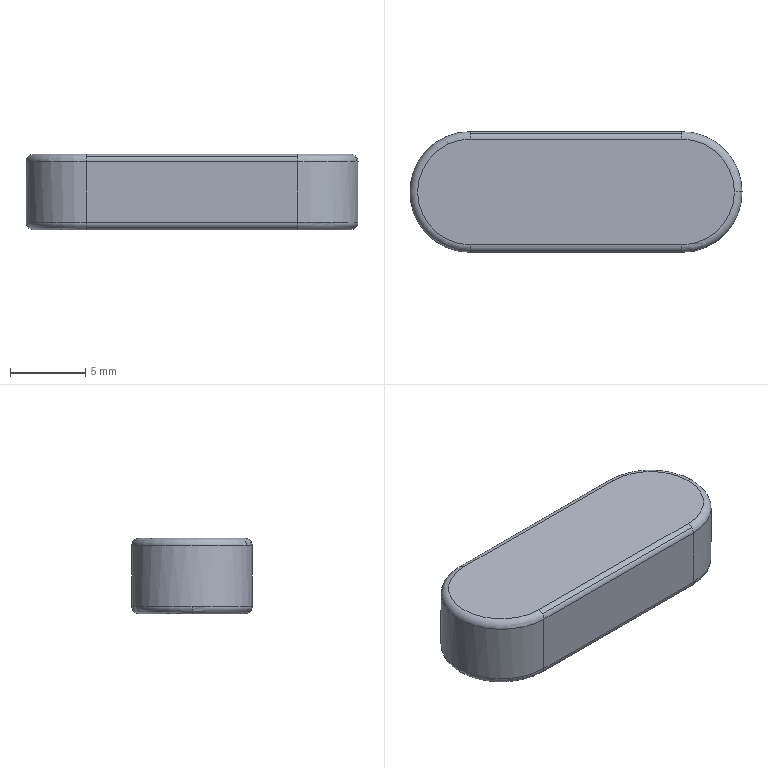Part | SolidWorks | features BaseBody 1 | 1 solid | 20 faces | box 22 x 8 x 5 mm | volume 805.702 mm3 | cylinder 10 | torus 6 | plane 4 | commonest cylinder face diameters 1 x8 8 x2
STEP:
#1=CARTESIAN_POINT('',(0.,-8.,-4.5));
#2=VERTEX_POINT('',#1);
#3=CARTESIAN_POINT('',(0.,-7.854,-4.854));
#4=VERTEX_POINT('',#3);
#5=CARTESIAN_POINT('',(0.,-7.5,-4.5));
#6=DIRECTION('',(1.,0.,0.));
#7=DIRECTION('',(0.,-1.,0.));
#8=AXIS2_PLACEMENT_3D('',#5,#6,#7);
#9=CIRCLE('',#8,0.5);
#10=EDGE_CURVE('',#2,#4,#9,.T.);
#11=ORIENTED_EDGE('',*,*,#10,.T.);
#12=CARTESIAN_POINT('',(14.,-7.854,-4.854));
#13=VERTEX_POINT('',#12);
#14=CARTESIAN_POINT('',(6.311,-7.854,-4.854));
#15=DIRECTION('',(1.,0.,0.));
#16=VECTOR('',#15,1000.);
#17=LINE('',#14,#16);
#18=EDGE_CURVE('',#4,#13,#17,.T.);
#19=ORIENTED_EDGE('',*,*,#18,.T.);
#20=CARTESIAN_POINT('',(14.,-8.,-4.5));
#21=VERTEX_POINT('',#20);
#22=CARTESIAN_POINT('',(14.,-7.5,-4.5));
#23=DIRECTION('',(-1.,0.,0.));
#24=DIRECTION('',(0.,0.,-1.));
#25=AXIS2_PLACEMENT_3D('',#22,#23,#24);
#26=CIRCLE('',#25,0.5);
#27=EDGE_CURVE('',#13,#21,#26,.T.);
#28=ORIENTED_EDGE('',*,*,#27,.T.);
#29=CARTESIAN_POINT('',(6.311,-8.,-4.5));
#30=DIRECTION('',(-1.,0.,0.));
#31=VECTOR('',#30,1000.);
#32=LINE('',#29,#31);
#33=EDGE_CURVE('',#21,#2,#32,.T.);
#34=ORIENTED_EDGE('',*,*,#33,.T.);
#35=EDGE_LOOP('',(#11,#19,#28,#34));
#36=FACE_OUTER_BOUND('',#35,.T.);
#37=CARTESIAN_POINT('',(6.311,-7.5,-4.5));
#38=DIRECTION('',(1.,0.,0.));
#39=DIRECTION('',(0.,-0.7071,-0.7071));
#40=AXIS2_PLACEMENT_3D('',#37,#38,#39);
#41=CYLINDRICAL_SURFACE('',#40,0.5);
#42=ADVANCED_FACE('',(#36),#41,.T.);
#43=CARTESIAN_POINT('',(-4.,-4.,-4.5));
#44=VERTEX_POINT('',#43);
#45=CARTESIAN_POINT('',(0.,-4.,-4.5));
#46=DIRECTION('',(0.,0.,-1.));
#47=DIRECTION('',(-1.,0.,0.));
#48=AXIS2_PLACEMENT_3D('',#45,#46,#47);
#49=CIRCLE('',#48,4.);
#50=EDGE_CURVE('',#2,#44,#49,.T.);
#51=ORIENTED_EDGE('',*,*,#50,.T.);
#52=CARTESIAN_POINT('',(-3.5,-4.,-5.));
#53=VERTEX_POINT('',#52);
#54=CARTESIAN_POINT('',(-3.5,-4.,-4.5));
#55=DIRECTION('',(0.,-1.,0.));
#56=DIRECTION('',(0.,0.,-1.));
#57=AXIS2_PLACEMENT_3D('',#54,#55,#56);
#58=CIRCLE('',#57,0.5);
#59=EDGE_CURVE('',#44,#53,#58,.T.);
#60=ORIENTED_EDGE('',*,*,#59,.T.);
#61=CARTESIAN_POINT('',(0.,-7.5,-5.));
#62=VERTEX_POINT('',#61);
#63=CARTESIAN_POINT('',(0.,-4.,-5.));
#64=DIRECTION('',(0.,0.,1.));
#65=DIRECTION('',(-1.,0.,0.));
#66=AXIS2_PLACEMENT_3D('',#63,#64,#65);
#67=CIRCLE('',#66,3.5);
#68=EDGE_CURVE('',#53,#62,#67,.T.);
#69=ORIENTED_EDGE('',*,*,#68,.T.);
#70=CARTESIAN_POINT('',(0.,-7.5,-4.5));
#71=DIRECTION('',(1.,0.,0.));
#72=DIRECTION('',(0.,-1.,0.));
#73=AXIS2_PLACEMENT_3D('',#70,#71,#72);
#74=CIRCLE('',#73,0.5);
#75=EDGE_CURVE('',#4,#62,#74,.T.);
#76=ORIENTED_EDGE('',*,*,#75,.F.);
#77=ORIENTED_EDGE('',*,*,#10,.F.);
#78=EDGE_LOOP('',(#51,#60,#69,#76,#77));
#79=FACE_OUTER_BOUND('',#78,.T.);
#80=CARTESIAN_POINT('',(0.,-4.,-4.5));
#81=DIRECTION('',(0.,0.,-1.));
#82=DIRECTION('',(-1.,0.,0.));
#83=AXIS2_PLACEMENT_3D('',#80,#81,#82);
#84=TOROIDAL_SURFACE('',#83,3.5,0.5);
#85=ADVANCED_FACE('',(#79),#84,.T.);
#86=CARTESIAN_POINT('',(14.,0.,-4.5));
#87=VERTEX_POINT('',#86);
#88=CARTESIAN_POINT('',(14.,-0.1464,-4.854));
#89=VERTEX_POINT('',#88);
#90=CARTESIAN_POINT('',(14.,-0.5,-4.5));
#91=DIRECTION('',(-1.,0.,0.));
#92=DIRECTION('',(0.,1.,0.));
#93=AXIS2_PLACEMENT_3D('',#90,#91,#92);
#94=CIRCLE('',#93,0.5);
#95=EDGE_CURVE('',#87,#89,#94,.T.);
#96=ORIENTED_EDGE('',*,*,#95,.T.);
#97=CARTESIAN_POINT('',(0.,-0.1464,-4.854));
#98=VERTEX_POINT('',#97);
#99=CARTESIAN_POINT('',(-0.6887,-0.1464,-4.854));
#100=DIRECTION('',(-1.,0.,0.));
#101=VECTOR('',#100,1000.);
#102=LINE('',#99,#101);
#103=EDGE_CURVE('',#89,#98,#102,.T.);
#104=ORIENTED_EDGE('',*,*,#103,.T.);
#105=CARTESIAN_POINT('',(0.,0.,-4.5));
#106=VERTEX_POINT('',#105);
#107=CARTESIAN_POINT('',(0.,-0.5,-4.5));
#108=DIRECTION('',(-1.,0.,0.));
#109=DIRECTION('',(0.,1.,0.));
#110=AXIS2_PLACEMENT_3D('',#107,#108,#109);
#111=CIRCLE('',#110,0.5);
#112=EDGE_CURVE('',#106,#98,#111,.T.);
#113=ORIENTED_EDGE('',*,*,#112,.F.);
#114=CARTESIAN_POINT('',(-0.6887,0.,-4.5));
#115=DIRECTION('',(1.,0.,0.));
#116=VECTOR('',#115,1000.);
#117=LINE('',#114,#116);
#118=EDGE_CURVE('',#106,#87,#117,.T.);
#119=ORIENTED_EDGE('',*,*,#118,.T.);
#120=EDGE_LOOP('',(#96,#104,#113,#119));
#121=FACE_OUTER_BOUND('',#120,.T.);
#122=CARTESIAN_POINT('',(-0.6887,-0.5,-4.5));
#123=DIRECTION('',(-1.,0.,0.));
#124=DIRECTION('',(0.,0.7071,-0.7071));
#125=AXIS2_PLACEMENT_3D('',#122,#123,#124);
#126=CYLINDRICAL_SURFACE('',#125,0.5);
#127=ADVANCED_FACE('',(#121),#126,.T.);
#128=CARTESIAN_POINT('',(0.,0.,-0.5));
#129=VERTEX_POINT('',#128);
#130=CARTESIAN_POINT('',(0.,-0.1464,-0.1464));
#131=VERTEX_POINT('',#130);
#132=CARTESIAN_POINT('',(0.,-0.5,-0.5));
#133=DIRECTION('',(1.,0.,0.));
#134=DIRECTION('',(0.,1.,0.));
#135=AXIS2_PLACEMENT_3D('',#132,#133,#134);
#136=CIRCLE('',#135,0.5);
#137=EDGE_CURVE('',#129,#131,#136,.T.);
#138=ORIENTED_EDGE('',*,*,#137,.T.);
#139=CARTESIAN_POINT('',(14.,-0.1464,-0.1464));
#140=VERTEX_POINT('',#139);
#141=CARTESIAN_POINT('',(-0.6887,-0.1464,-0.1464));
#142=DIRECTION('',(1.,0.,0.));
#143=VECTOR('',#142,1000.);
#144=LINE('',#141,#143);
#145=EDGE_CURVE('',#131,#140,#144,.T.);
#146=ORIENTED_EDGE('',*,*,#145,.T.);
#147=CARTESIAN_POINT('',(14.,0.,-0.5));
#148=VERTEX_POINT('',#147);
#149=CARTESIAN_POINT('',(14.,-0.5,-0.5));
#150=DIRECTION('',(-1.,0.,0.));
#151=DIRECTION('',(0.,0.,1.));
#152=AXIS2_PLACEMENT_3D('',#149,#150,#151);
#153=CIRCLE('',#152,0.5);
#154=EDGE_CURVE('',#140,#148,#153,.T.);
#155=ORIENTED_EDGE('',*,*,#154,.T.);
#156=CARTESIAN_POINT('',(-0.6887,0.,-0.5));
#157=DIRECTION('',(-1.,0.,0.));
#158=VECTOR('',#157,1000.);
#159=LINE('',#156,#158);
#160=EDGE_CURVE('',#148,#129,#159,.T.);
#161=ORIENTED_EDGE('',*,*,#160,.T.);
#162=EDGE_LOOP('',(#138,#146,#155,#161));
#163=FACE_OUTER_BOUND('',#162,.T.);
#164=CARTESIAN_POINT('',(-0.6887,-0.5,-0.5));
#165=DIRECTION('',(1.,0.,0.));
#166=DIRECTION('',(0.,0.7071,0.7071));
#167=AXIS2_PLACEMENT_3D('',#164,#165,#166);
#168=CYLINDRICAL_SURFACE('',#167,0.5);
#169=ADVANCED_FACE('',(#163),#168,.T.);
#170=CARTESIAN_POINT('',(14.,-8.,-0.5));
#171=VERTEX_POINT('',#170);
#172=CARTESIAN_POINT('',(14.,-7.854,-0.1464));
#173=VERTEX_POINT('',#172);
#174=CARTESIAN_POINT('',(14.,-7.5,-0.5));
#175=DIRECTION('',(-1.,0.,0.));
#176=DIRECTION('',(0.,-1.,0.));
#177=AXIS2_PLACEMENT_3D('',#174,#175,#176);
#178=CIRCLE('',#177,0.5);
#179=EDGE_CURVE('',#171,#173,#178,.T.);
#180=ORIENTED_EDGE('',*,*,#179,.T.);
#181=CARTESIAN_POINT('',(0.,-7.854,-0.1464));
#182=VERTEX_POINT('',#181);
#183=CARTESIAN_POINT('',(6.311,-7.854,-0.1464));
#184=DIRECTION('',(-1.,0.,0.));
#185=VECTOR('',#184,1000.);
#186=LINE('',#183,#185);
#187=EDGE_CURVE('',#173,#182,#186,.T.);
#188=ORIENTED_EDGE('',*,*,#187,.T.);
#189=CARTESIAN_POINT('',(0.,-8.,-0.5));
#190=VERTEX_POINT('',#189);
#191=CARTESIAN_POINT('',(0.,-7.5,-0.5));
#192=DIRECTION('',(-1.,0.,0.));
#193=DIRECTION('',(0.,-1.,0.));
#194=AXIS2_PLACEMENT_3D('',#191,#192,#193);
#195=CIRCLE('',#194,0.5);
#196=EDGE_CURVE('',#190,#182,#195,.T.);
#197=ORIENTED_EDGE('',*,*,#196,.F.);
#198=CARTESIAN_POINT('',(6.311,-8.,-0.5));
#199=DIRECTION('',(1.,0.,0.));
#200=VECTOR('',#199,1000.);
#201=LINE('',#198,#200);
#202=EDGE_CURVE('',#190,#171,#201,.T.);
#203=ORIENTED_EDGE('',*,*,#202,.T.);
#204=EDGE_LOOP('',(#180,#188,#197,#203));
#205=FACE_OUTER_BOUND('',#204,.T.);
#206=CARTESIAN_POINT('',(6.311,-7.5,-0.5));
#207=DIRECTION('',(-1.,0.,0.));
#208=DIRECTION('',(0.,-0.7071,0.7071));
#209=AXIS2_PLACEMENT_3D('',#206,#207,#208);
#210=CYLINDRICAL_SURFACE('',#209,0.5);
#211=ADVANCED_FACE('',(#205),#210,.T.);
#212=CARTESIAN_POINT('',(18.,-4.,-0.5));
#213=VERTEX_POINT('',#212);
#214=CARTESIAN_POINT('',(14.,-4.,-0.5));
#215=DIRECTION('',(0.,0.,1.));
#216=DIRECTION('',(1.,0.,0.));
#217=AXIS2_PLACEMENT_3D('',#214,#215,#216);
#218=CIRCLE('',#217,4.);
#219=EDGE_CURVE('',#171,#213,#218,.T.);
#220=ORIENTED_EDGE('',*,*,#219,.T.);
#221=CARTESIAN_POINT('',(17.5,-4.,0.));
#222=VERTEX_POINT('',#221);
#223=CARTESIAN_POINT('',(17.5,-4.,-0.5));
#224=DIRECTION('',(0.,-1.,0.));
#225=DIRECTION('',(0.,0.,-1.));
#226=AXIS2_PLACEMENT_3D('',#223,#224,#225);
#227=CIRCLE('',#226,0.5);
#228=EDGE_CURVE('',#213,#222,#227,.T.);
#229=ORIENTED_EDGE('',*,*,#228,.T.);
#230=CARTESIAN_POINT('',(14.,-7.5,0.));
#231=VERTEX_POINT('',#230);
#232=CARTESIAN_POINT('',(14.,-4.,0.));
#233=DIRECTION('',(0.,0.,-1.));
#234=DIRECTION('',(1.,0.,0.));
#235=AXIS2_PLACEMENT_3D('',#232,#233,#234);
#236=CIRCLE('',#235,3.5);
#237=EDGE_CURVE('',#222,#231,#236,.T.);
#238=ORIENTED_EDGE('',*,*,#237,.T.);
#239=CARTESIAN_POINT('',(14.,-7.5,-0.5));
#240=DIRECTION('',(-1.,0.,0.));
#241=DIRECTION('',(0.,-1.,0.));
#242=AXIS2_PLACEMENT_3D('',#239,#240,#241);
#243=CIRCLE('',#242,0.5);
#244=EDGE_CURVE('',#173,#231,#243,.T.);
#245=ORIENTED_EDGE('',*,*,#244,.F.);
#246=ORIENTED_EDGE('',*,*,#179,.F.);
#247=EDGE_LOOP('',(#220,#229,#238,#245,#246));
#248=FACE_OUTER_BOUND('',#247,.T.);
#249=CARTESIAN_POINT('',(14.,-4.,-0.5));
#250=DIRECTION('',(0.,0.,1.));
#251=DIRECTION('',(1.,0.,0.));
#252=AXIS2_PLACEMENT_3D('',#249,#250,#251);
#253=TOROIDAL_SURFACE('',#252,3.5,0.5);
#254=ADVANCED_FACE('',(#248),#253,.T.);
#255=CARTESIAN_POINT('',(14.,-7.5,-5.));
#256=VERTEX_POINT('',#255);
#257=CARTESIAN_POINT('',(14.,-7.5,-4.5));
#258=DIRECTION('',(-1.,0.,0.));
#259=DIRECTION('',(0.,0.,-1.));
#260=AXIS2_PLACEMENT_3D('',#257,#258,#259);
#261=CIRCLE('',#260,0.5);
#262=EDGE_CURVE('',#256,#13,#261,.T.);
#263=ORIENTED_EDGE('',*,*,#262,.F.);
#264=CARTESIAN_POINT('',(14.,-0.5,-5.));
#265=VERTEX_POINT('',#264);
#266=CARTESIAN_POINT('',(14.,-4.,-5.));
#267=DIRECTION('',(0.,0.,1.));
#268=DIRECTION('',(1.,0.,0.));
#269=AXIS2_PLACEMENT_3D('',#266,#267,#268);
#270=CIRCLE('',#269,3.5);
#271=EDGE_CURVE('',#256,#265,#270,.T.);
#272=ORIENTED_EDGE('',*,*,#271,.T.);
#273=CARTESIAN_POINT('',(14.,-0.5,-4.5));
#274=DIRECTION('',(-1.,0.,0.));
#275=DIRECTION('',(0.,1.,0.));
#276=AXIS2_PLACEMENT_3D('',#273,#274,#275);
#277=CIRCLE('',#276,0.5);
#278=EDGE_CURVE('',#89,#265,#277,.T.);
#279=ORIENTED_EDGE('',*,*,#278,.F.);
#280=ORIENTED_EDGE('',*,*,#95,.F.);
#281=CARTESIAN_POINT('',(14.,-4.,-4.5));
#282=DIRECTION('',(0.,0.,-1.));
#283=DIRECTION('',(1.,0.,0.));
#284=AXIS2_PLACEMENT_3D('',#281,#282,#283);
#285=CIRCLE('',#284,4.);
#286=EDGE_CURVE('',#87,#21,#285,.T.);
#287=ORIENTED_EDGE('',*,*,#286,.T.);
#288=ORIENTED_EDGE('',*,*,#27,.F.);
#289=EDGE_LOOP('',(#263,#272,#279,#280,#287,#288));
#290=FACE_OUTER_BOUND('',#289,.T.);
#291=CARTESIAN_POINT('',(14.,-4.,-4.5));
#292=DIRECTION('',(0.,0.,-1.));
#293=DIRECTION('',(-1.,0.,0.));
#294=AXIS2_PLACEMENT_3D('',#291,#292,#293);
#295=TOROIDAL_SURFACE('',#294,3.5,0.5);
#296=ADVANCED_FACE('',(#290),#295,.T.);
#297=ORIENTED_EDGE('',*,*,#50,.F.);
#298=CARTESIAN_POINT('',(0.,-8.,0.));
#299=DIRECTION('',(0.,0.,-1.));
#300=VECTOR('',#299,1000.);
#301=LINE('',#298,#300);
#302=EDGE_CURVE('',#190,#2,#301,.T.);
#303=ORIENTED_EDGE('',*,*,#302,.F.);
#304=CARTESIAN_POINT('',(0.,-4.,-0.5));
#305=DIRECTION('',(0.,0.,1.));
#306=DIRECTION('',(-1.,0.,0.));
#307=AXIS2_PLACEMENT_3D('',#304,#305,#306);
#308=CIRCLE('',#307,4.);
#309=EDGE_CURVE('',#129,#190,#308,.T.);
#310=ORIENTED_EDGE('',*,*,#309,.F.);
#311=CARTESIAN_POINT('',(0.,0.,0.));
#312=DIRECTION('',(0.,0.,-1.));
#313=VECTOR('',#312,1000.);
#314=LINE('',#311,#313);
#315=EDGE_CURVE('',#129,#106,#314,.T.);
#316=ORIENTED_EDGE('',*,*,#315,.T.);
#317=CARTESIAN_POINT('',(0.,-4.,-4.5));
#318=DIRECTION('',(0.,0.,-1.));
#319=DIRECTION('',(-1.,0.,0.));
#320=AXIS2_PLACEMENT_3D('',#317,#318,#319);
#321=CIRCLE('',#320,4.);
#322=EDGE_CURVE('',#44,#106,#321,.T.);
#323=ORIENTED_EDGE('',*,*,#322,.F.);
#324=EDGE_LOOP('',(#297,#303,#310,#316,#323));
#325=FACE_OUTER_BOUND('',#324,.T.);
#326=CARTESIAN_POINT('',(0.,-4.,0.));
#327=DIRECTION('',(0.,0.,1.));
#328=DIRECTION('',(0.,1.,0.));
#329=AXIS2_PLACEMENT_3D('',#326,#327,#328);
#330=CYLINDRICAL_SURFACE('',#329,4.);
#331=ADVANCED_FACE('',(#325),#330,.T.);
#332=ORIENTED_EDGE('',*,*,#33,.F.);
#333=CARTESIAN_POINT('',(14.,-8.,0.));
#334=DIRECTION('',(0.,0.,-1.));
#335=VECTOR('',#334,1000.);
#336=LINE('',#333,#335);
#337=EDGE_CURVE('',#171,#21,#336,.T.);
#338=ORIENTED_EDGE('',*,*,#337,.F.);
#339=ORIENTED_EDGE('',*,*,#202,.F.);
#340=ORIENTED_EDGE('',*,*,#302,.T.);
#341=EDGE_LOOP('',(#332,#338,#339,#340));
#342=FACE_OUTER_BOUND('',#341,.T.);
#343=CARTESIAN_POINT('',(14.,-8.,0.));
#344=DIRECTION('',(0.,-1.,0.));
#345=DIRECTION('',(-1.,0.,0.));
#346=AXIS2_PLACEMENT_3D('',#343,#344,#345);
#347=PLANE('',#346);
#348=ADVANCED_FACE('',(#342),#347,.T.);
#349=CARTESIAN_POINT('',(6.311,-7.5,-5.));
#350=DIRECTION('',(1.,0.,0.));
#351=VECTOR('',#350,1000.);
#352=LINE('',#349,#351);
#353=EDGE_CURVE('',#62,#256,#352,.T.);
#354=ORIENTED_EDGE('',*,*,#353,.F.);
#355=ORIENTED_EDGE('',*,*,#68,.F.);
#356=CARTESIAN_POINT('',(0.,-0.5,-5.));
#357=VERTEX_POINT('',#356);
#358=CARTESIAN_POINT('',(0.,-4.,-5.));
#359=DIRECTION('',(0.,0.,1.));
#360=DIRECTION('',(-1.,0.,0.));
#361=AXIS2_PLACEMENT_3D('',#358,#359,#360);
#362=CIRCLE('',#361,3.5);
#363=EDGE_CURVE('',#357,#53,#362,.T.);
#364=ORIENTED_EDGE('',*,*,#363,.F.);
#365=CARTESIAN_POINT('',(-0.6887,-0.5,-5.));
#366=DIRECTION('',(-1.,0.,0.));
#367=VECTOR('',#366,1000.);
#368=LINE('',#365,#367);
#369=EDGE_CURVE('',#265,#357,#368,.T.);
#370=ORIENTED_EDGE('',*,*,#369,.F.);
#371=ORIENTED_EDGE('',*,*,#271,.F.);
#372=EDGE_LOOP('',(#354,#355,#364,#370,#371));
#373=FACE_OUTER_BOUND('',#372,.T.);
#374=CARTESIAN_POINT('',(-1.377,-4.,-5.));
#375=DIRECTION('',(0.,0.,1.));
#376=DIRECTION('',(1.,0.,0.));
#377=AXIS2_PLACEMENT_3D('',#374,#375,#376);
#378=PLANE('',#377);
#379=ADVANCED_FACE('',(#373),#378,.F.);
#380=ORIENTED_EDGE('',*,*,#196,.T.);
#381=CARTESIAN_POINT('',(0.,-7.5,0.));
#382=VERTEX_POINT('',#381);
#383=CARTESIAN_POINT('',(0.,-7.5,-0.5));
#384=DIRECTION('',(-1.,0.,0.));
#385=DIRECTION('',(0.,-1.,0.));
#386=AXIS2_PLACEMENT_3D('',#383,#384,#385);
#387=CIRCLE('',#386,0.5);
#388=EDGE_CURVE('',#182,#382,#387,.T.);
#389=ORIENTED_EDGE('',*,*,#388,.T.);
#390=CARTESIAN_POINT('',(0.,-0.5,0.));
#391=VERTEX_POINT('',#390);
#392=CARTESIAN_POINT('',(0.,-4.,0.));
#393=DIRECTION('',(0.,0.,-1.));
#394=DIRECTION('',(-1.,0.,0.));
#395=AXIS2_PLACEMENT_3D('',#392,#393,#394);
#396=CIRCLE('',#395,3.5);
#397=EDGE_CURVE('',#382,#391,#396,.T.);
#398=ORIENTED_EDGE('',*,*,#397,.T.);
#399=CARTESIAN_POINT('',(0.,-0.5,-0.5));
#400=DIRECTION('',(1.,0.,0.));
#401=DIRECTION('',(0.,1.,0.));
#402=AXIS2_PLACEMENT_3D('',#399,#400,#401);
#403=CIRCLE('',#402,0.5);
#404=EDGE_CURVE('',#131,#391,#403,.T.);
#405=ORIENTED_EDGE('',*,*,#404,.F.);
#406=ORIENTED_EDGE('',*,*,#137,.F.);
#407=ORIENTED_EDGE('',*,*,#309,.T.);
#408=EDGE_LOOP('',(#380,#389,#398,#405,#406,#407));
#409=FACE_OUTER_BOUND('',#408,.T.);
#410=CARTESIAN_POINT('',(0.,-4.,-0.5));
#411=DIRECTION('',(0.,0.,1.));
#412=DIRECTION('',(1.,0.,0.));
#413=AXIS2_PLACEMENT_3D('',#410,#411,#412);
#414=TOROIDAL_SURFACE('',#413,3.5,0.5);
#415=ADVANCED_FACE('',(#409),#414,.T.);
#416=ORIENTED_EDGE('',*,*,#118,.F.);
#417=ORIENTED_EDGE('',*,*,#315,.F.);
#418=ORIENTED_EDGE('',*,*,#160,.F.);
#419=CARTESIAN_POINT('',(14.,0.,0.));
#420=DIRECTION('',(0.,0.,-1.));
#421=VECTOR('',#420,1000.);
#422=LINE('',#419,#421);
#423=EDGE_CURVE('',#148,#87,#422,.T.);
#424=ORIENTED_EDGE('',*,*,#423,.T.);
#425=EDGE_LOOP('',(#416,#417,#418,#424));
#426=FACE_OUTER_BOUND('',#425,.T.);
#427=CARTESIAN_POINT('',(0.,0.,0.));
#428=DIRECTION('',(0.,1.,0.));
#429=DIRECTION('',(1.,0.,0.));
#430=AXIS2_PLACEMENT_3D('',#427,#428,#429);
#431=PLANE('',#430);
#432=ADVANCED_FACE('',(#426),#431,.T.);
#433=CARTESIAN_POINT('',(14.,-0.5,0.));
#434=VERTEX_POINT('',#433);
#435=CARTESIAN_POINT('',(-0.6887,-0.5,0.));
#436=DIRECTION('',(1.,0.,0.));
#437=VECTOR('',#436,1000.);
#438=LINE('',#435,#437);
#439=EDGE_CURVE('',#391,#434,#438,.T.);
#440=ORIENTED_EDGE('',*,*,#439,.F.);
#441=ORIENTED_EDGE('',*,*,#397,.F.);
#442=CARTESIAN_POINT('',(6.311,-7.5,0.));
#443=DIRECTION('',(-1.,0.,0.));
#444=VECTOR('',#443,1000.);
#445=LINE('',#442,#444);
#446=EDGE_CURVE('',#231,#382,#445,.T.);
#447=ORIENTED_EDGE('',*,*,#446,.F.);
#448=ORIENTED_EDGE('',*,*,#237,.F.);
#449=CARTESIAN_POINT('',(14.,-4.,0.));
#450=DIRECTION('',(0.,0.,-1.));
#451=DIRECTION('',(1.,0.,0.));
#452=AXIS2_PLACEMENT_3D('',#449,#450,#451);
#453=CIRCLE('',#452,3.5);
#454=EDGE_CURVE('',#434,#222,#453,.T.);
#455=ORIENTED_EDGE('',*,*,#454,.F.);
#456=EDGE_LOOP('',(#440,#441,#447,#448,#455));
#457=FACE_OUTER_BOUND('',#456,.T.);
#458=CARTESIAN_POINT('',(-1.377,-4.,0.));
#459=DIRECTION('',(0.,0.,1.));
#460=DIRECTION('',(1.,0.,0.));
#461=AXIS2_PLACEMENT_3D('',#458,#459,#460);
#462=PLANE('',#461);
#463=ADVANCED_FACE('',(#457),#462,.T.);
#464=ORIENTED_EDGE('',*,*,#286,.F.);
#465=ORIENTED_EDGE('',*,*,#423,.F.);
#466=CARTESIAN_POINT('',(14.,-4.,-0.5));
#467=DIRECTION('',(0.,0.,1.));
#468=DIRECTION('',(1.,0.,0.));
#469=AXIS2_PLACEMENT_3D('',#466,#467,#468);
#470=CIRCLE('',#469,4.);
#471=EDGE_CURVE('',#213,#148,#470,.T.);
#472=ORIENTED_EDGE('',*,*,#471,.F.);
#473=ORIENTED_EDGE('',*,*,#219,.F.);
#474=ORIENTED_EDGE('',*,*,#337,.T.);
#475=EDGE_LOOP('',(#464,#465,#472,#473,#474));
#476=FACE_OUTER_BOUND('',#475,.T.);
#477=CARTESIAN_POINT('',(14.,-4.,0.));
#478=DIRECTION('',(0.,0.,1.));
#479=DIRECTION('',(0.,-1.,0.));
#480=AXIS2_PLACEMENT_3D('',#477,#478,#479);
#481=CYLINDRICAL_SURFACE('',#480,4.);
#482=ADVANCED_FACE('',(#476),#481,.T.);
#483=ORIENTED_EDGE('',*,*,#228,.F.);
#484=ORIENTED_EDGE('',*,*,#471,.T.);
#485=ORIENTED_EDGE('',*,*,#154,.F.);
#486=CARTESIAN_POINT('',(14.,-0.5,-0.5));
#487=DIRECTION('',(-1.,0.,0.));
#488=DIRECTION('',(0.,0.,1.));
#489=AXIS2_PLACEMENT_3D('',#486,#487,#488);
#490=CIRCLE('',#489,0.5);
#491=EDGE_CURVE('',#434,#140,#490,.T.);
#492=ORIENTED_EDGE('',*,*,#491,.F.);
#493=ORIENTED_EDGE('',*,*,#454,.T.);
#494=EDGE_LOOP('',(#483,#484,#485,#492,#493));
#495=FACE_OUTER_BOUND('',#494,.T.);
#496=CARTESIAN_POINT('',(14.,-4.,-0.5));
#497=DIRECTION('',(0.,0.,1.));
#498=DIRECTION('',(1.,0.,0.));
#499=AXIS2_PLACEMENT_3D('',#496,#497,#498);
#500=TOROIDAL_SURFACE('',#499,3.5,0.5);
#501=ADVANCED_FACE('',(#495),#500,.T.);
#502=ORIENTED_EDGE('',*,*,#187,.F.);
#503=ORIENTED_EDGE('',*,*,#244,.T.);
#504=ORIENTED_EDGE('',*,*,#446,.T.);
#505=ORIENTED_EDGE('',*,*,#388,.F.);
#506=EDGE_LOOP('',(#502,#503,#504,#505));
#507=FACE_OUTER_BOUND('',#506,.T.);
#508=CARTESIAN_POINT('',(6.311,-7.5,-0.5));
#509=DIRECTION('',(-1.,0.,0.));
#510=DIRECTION('',(0.,-0.7071,0.7071));
#511=AXIS2_PLACEMENT_3D('',#508,#509,#510);
#512=CYLINDRICAL_SURFACE('',#511,0.5);
#513=ADVANCED_FACE('',(#507),#512,.T.);
#514=ORIENTED_EDGE('',*,*,#145,.F.);
#515=ORIENTED_EDGE('',*,*,#404,.T.);
#516=ORIENTED_EDGE('',*,*,#439,.T.);
#517=ORIENTED_EDGE('',*,*,#491,.T.);
#518=EDGE_LOOP('',(#514,#515,#516,#517));
#519=FACE_OUTER_BOUND('',#518,.T.);
#520=CARTESIAN_POINT('',(-0.6887,-0.5,-0.5));
#521=DIRECTION('',(1.,0.,0.));
#522=DIRECTION('',(0.,0.7071,0.7071));
#523=AXIS2_PLACEMENT_3D('',#520,#521,#522);
#524=CYLINDRICAL_SURFACE('',#523,0.5);
#525=ADVANCED_FACE('',(#519),#524,.T.);
#526=ORIENTED_EDGE('',*,*,#103,.F.);
#527=ORIENTED_EDGE('',*,*,#278,.T.);
#528=ORIENTED_EDGE('',*,*,#369,.T.);
#529=CARTESIAN_POINT('',(0.,-0.5,-4.5));
#530=DIRECTION('',(-1.,0.,0.));
#531=DIRECTION('',(0.,1.,0.));
#532=AXIS2_PLACEMENT_3D('',#529,#530,#531);
#533=CIRCLE('',#532,0.5);
#534=EDGE_CURVE('',#98,#357,#533,.T.);
#535=ORIENTED_EDGE('',*,*,#534,.F.);
#536=EDGE_LOOP('',(#526,#527,#528,#535));
#537=FACE_OUTER_BOUND('',#536,.T.);
#538=CARTESIAN_POINT('',(-0.6887,-0.5,-4.5));
#539=DIRECTION('',(-1.,0.,0.));
#540=DIRECTION('',(0.,0.7071,-0.7071));
#541=AXIS2_PLACEMENT_3D('',#538,#539,#540);
#542=CYLINDRICAL_SURFACE('',#541,0.5);
#543=ADVANCED_FACE('',(#537),#542,.T.);
#544=ORIENTED_EDGE('',*,*,#59,.F.);
#545=ORIENTED_EDGE('',*,*,#322,.T.);
#546=ORIENTED_EDGE('',*,*,#112,.T.);
#547=ORIENTED_EDGE('',*,*,#534,.T.);
#548=ORIENTED_EDGE('',*,*,#363,.T.);
#549=EDGE_LOOP('',(#544,#545,#546,#547,#548));
#550=FACE_OUTER_BOUND('',#549,.T.);
#551=CARTESIAN_POINT('',(0.,-4.,-4.5));
#552=DIRECTION('',(0.,0.,-1.));
#553=DIRECTION('',(-1.,0.,0.));
#554=AXIS2_PLACEMENT_3D('',#551,#552,#553);
#555=TOROIDAL_SURFACE('',#554,3.5,0.5);
#556=ADVANCED_FACE('',(#550),#555,.T.);
#557=ORIENTED_EDGE('',*,*,#18,.F.);
#558=ORIENTED_EDGE('',*,*,#75,.T.);
#559=ORIENTED_EDGE('',*,*,#353,.T.);
#560=ORIENTED_EDGE('',*,*,#262,.T.);
#561=EDGE_LOOP('',(#557,#558,#559,#560));
#562=FACE_OUTER_BOUND('',#561,.T.);
#563=CARTESIAN_POINT('',(6.311,-7.5,-4.5));
#564=DIRECTION('',(1.,0.,0.));
#565=DIRECTION('',(0.,-0.7071,-0.7071));
#566=AXIS2_PLACEMENT_3D('',#563,#564,#565);
#567=CYLINDRICAL_SURFACE('',#566,0.5);
#568=ADVANCED_FACE('',(#562),#567,.T.);
#569=CLOSED_SHELL('',(#42,#85,#127,#169,#211,#254,#296,#331,#348,#379,#415,#432,#463,#482,#501,#513,#525,#543,#556,#568));
#570=MANIFOLD_SOLID_BREP('',#569);
#571=CARTESIAN_POINT('',(0.,0.,0.));
#572=DIRECTION('',(0.,0.,1.));
#573=DIRECTION('',(1.,0.,0.));
#574=AXIS2_PLACEMENT_3D('',#571,#572,#573);
#575=(LENGTH_UNIT()NAMED_UNIT(*)SI_UNIT(.MILLI.,.METRE.));
#576=UNCERTAINTY_MEASURE_WITH_UNIT(LENGTH_MEASURE(0.00001),#575,'','');
#577=(NAMED_UNIT(*)PLANE_ANGLE_UNIT()SI_UNIT($,.RADIAN.));
#578=(NAMED_UNIT(*)SI_UNIT($,.STERADIAN.)SOLID_ANGLE_UNIT());
#579=(GEOMETRIC_REPRESENTATION_CONTEXT(3)GLOBAL_UNCERTAINTY_ASSIGNED_CONTEXT((#576))GLOBAL_UNIT_ASSIGNED_CONTEXT((#575,#577,#578))REPRESENTATION_CONTEXT('',''));
#580=ADVANCED_BREP_SHAPE_REPRESENTATION('',(#570,#574),#579);